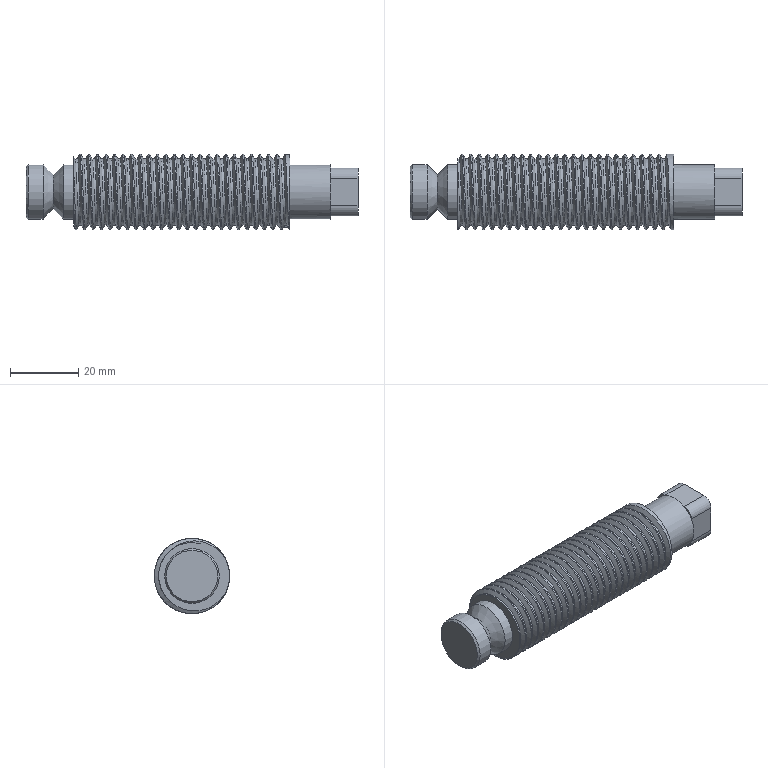Part | NX | features DATUM_CSYS 3, SKETCH 2, BLEND 1, CHAMFER 1, EXTRUDE 1, SWP104 1, THREADS 1 | 1 solid | 31 faces | box 97 x 22 x 22 mm | volume 27588 mm3 | plane 17 | cylinder 9 | cone 3 | spline 2 | commonest cylinder face diameters 6 x4 16 x3 19.5 x1 22 x1